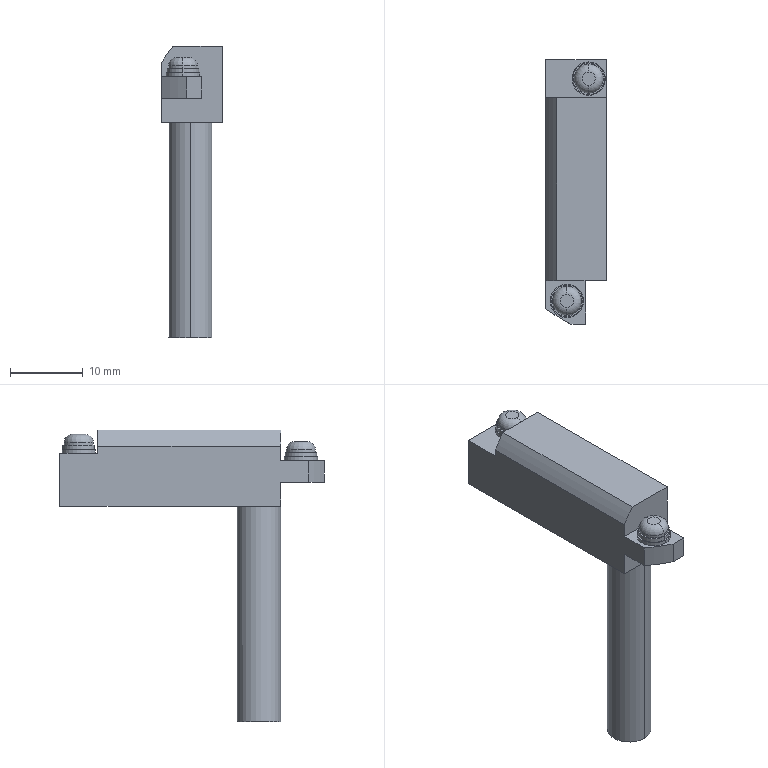Part | STEP file | Guide wheel mechanism revised.sldasm-Part-317 | 2 solids | 40 faces | box 8.3 x 36.4 x 40.2 mm | volume 3466 mm3 | plane 20 | cylinder 16 | torus 4 | commonest cylinder face diameters 4 x4 4.35 x4 4.6 x4 6 x2 32 x1 47 x1